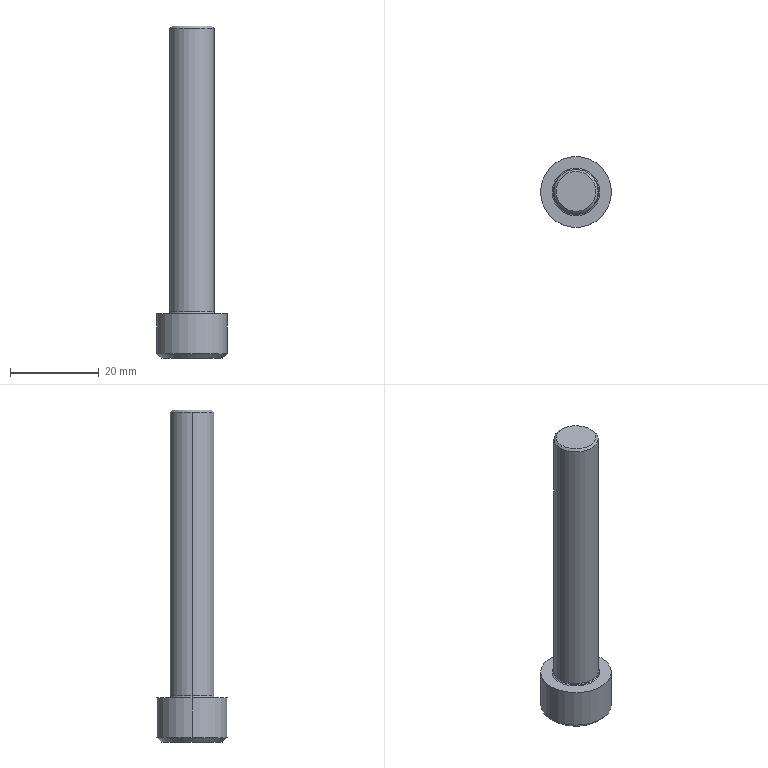Part | Creo | 1 solid | 23 faces | box 16 x 16 x 75 mm | volume 6754 mm3 | plane 9 | cone 6 | cylinder 4 | torus 4 | commonest cylinder face diameters 10 x2 16 x2
STEP:
#1=CARTESIAN_POINT('',(232.817,-87.997,-4.));
#2=VERTEX_POINT('',#1);
#3=CARTESIAN_POINT('',(235.126,-83.997,-4.));
#4=VERTEX_POINT('',#3);
#5=CARTESIAN_POINT('',(232.817,-87.997,-4.));
#6=CARTESIAN_POINT('',(232.943,-87.779,-3.928));
#7=CARTESIAN_POINT('',(233.195,-87.342,-3.799));
#8=CARTESIAN_POINT('',(233.581,-86.674,-3.673));
#9=CARTESIAN_POINT('',(233.971,-85.999,-3.628));
#10=CARTESIAN_POINT('',(234.362,-85.321,-3.672));
#11=CARTESIAN_POINT('',(234.747,-84.654,-3.799));
#12=CARTESIAN_POINT('',(235.,-84.215,-3.927));
#13=CARTESIAN_POINT('',(235.126,-83.997,-4.));
#14=B_SPLINE_CURVE_WITH_KNOTS('',3,(#5,#6,#7,#8,#9,#10,#11,#12,#13),.UNSPECIFIED.,.F.,.F.,(4,1,1,1,1,1,4),(0.,0.1667,0.3333,0.5,0.6667,0.8333,1.),.UNSPECIFIED.);
#15=EDGE_CURVE('',#2,#4,#14,.T.);
#16=ORIENTED_EDGE('',*,*,#15,.F.);
#17=CARTESIAN_POINT('',(237.436,-87.997,-1.333));
#18=VERTEX_POINT('',#17);
#19=CARTESIAN_POINT('',(237.436,-87.997,-1.333));
#20=DIRECTION('',(-0.866,0.,-0.5));
#21=VECTOR('',#20,5.333);
#22=LINE('',#19,#21);
#23=EDGE_CURVE('',#18,#2,#22,.T.);
#24=ORIENTED_EDGE('',*,*,#23,.F.);
#25=CARTESIAN_POINT('',(242.055,-87.997,-4.));
#26=VERTEX_POINT('',#25);
#27=CARTESIAN_POINT('',(237.436,-87.997,-1.333));
#28=DIRECTION('',(0.866,0.,-0.5));
#29=VECTOR('',#28,5.333);
#30=LINE('',#27,#29);
#31=EDGE_CURVE('',#18,#26,#30,.T.);
#32=ORIENTED_EDGE('',*,*,#31,.T.);
#33=CARTESIAN_POINT('',(239.745,-83.997,-4.));
#34=VERTEX_POINT('',#33);
#35=CARTESIAN_POINT('',(239.745,-83.997,-4.));
#36=CARTESIAN_POINT('',(239.871,-84.214,-3.928));
#37=CARTESIAN_POINT('',(240.123,-84.651,-3.799));
#38=CARTESIAN_POINT('',(240.509,-85.32,-3.673));
#39=CARTESIAN_POINT('',(240.899,-85.995,-3.628));
#40=CARTESIAN_POINT('',(241.29,-86.673,-3.672));
#41=CARTESIAN_POINT('',(241.675,-87.34,-3.799));
#42=CARTESIAN_POINT('',(241.929,-87.778,-3.927));
#43=CARTESIAN_POINT('',(242.055,-87.997,-4.));
#44=B_SPLINE_CURVE_WITH_KNOTS('',3,(#35,#36,#37,#38,#39,#40,#41,#42,#43),.UNSPECIFIED.,.F.,.F.,(4,1,1,1,1,1,4),(0.,0.1667,0.3333,0.5,0.6667,0.8333,1.),.UNSPECIFIED.);
#45=EDGE_CURVE('',#34,#26,#44,.T.);
#46=ORIENTED_EDGE('',*,*,#45,.F.);
#47=CARTESIAN_POINT('',(235.126,-83.997,-4.));
#48=CARTESIAN_POINT('',(235.376,-83.997,-3.928));
#49=CARTESIAN_POINT('',(235.88,-83.997,-3.8));
#50=CARTESIAN_POINT('',(236.654,-83.997,-3.673));
#51=CARTESIAN_POINT('',(237.435,-83.997,-3.628));
#52=CARTESIAN_POINT('',(238.215,-83.997,-3.672));
#53=CARTESIAN_POINT('',(238.988,-83.997,-3.799));
#54=CARTESIAN_POINT('',(239.494,-83.997,-3.927));
#55=CARTESIAN_POINT('',(239.745,-83.997,-4.));
#56=B_SPLINE_CURVE_WITH_KNOTS('',3,(#47,#48,#49,#50,#51,#52,#53,#54,#55),.UNSPECIFIED.,.F.,.F.,(4,1,1,1,1,1,4),(0.,0.1667,0.3333,0.5,0.6667,0.8333,1.),.UNSPECIFIED.);
#57=EDGE_CURVE('',#4,#34,#56,.T.);
#58=ORIENTED_EDGE('',*,*,#57,.F.);
#59=EDGE_LOOP('',(#16,#24,#32,#46,#58));
#60=FACE_OUTER_BOUND('',#59,.F.);
#61=CARTESIAN_POINT('',(237.436,-87.997,-2.693));
#62=DIRECTION('',(0.,0.,-1.));
#63=DIRECTION('',(-1.,0.,0.));
#64=AXIS2_PLACEMENT_3D('',#61,#62,#63);
#65=CONICAL_SURFACE('',#64,2.356,60.);
#66=ADVANCED_FACE('',(#60),#65,.F.);
#67=CARTESIAN_POINT('',(235.126,-83.997,-9.));
#68=VERTEX_POINT('',#67);
#69=CARTESIAN_POINT('',(232.817,-87.997,-9.));
#70=VERTEX_POINT('',#69);
#71=CARTESIAN_POINT('',(235.126,-83.997,-9.));
#72=DIRECTION('',(-0.5,-0.866,0.));
#73=VECTOR('',#72,4.619);
#74=LINE('',#71,#73);
#75=EDGE_CURVE('',#68,#70,#74,.T.);
#76=ORIENTED_EDGE('',*,*,#75,.T.);
#77=CARTESIAN_POINT('',(232.817,-87.997,-9.));
#78=DIRECTION('',(0.,0.,1.));
#79=VECTOR('',#78,5.);
#80=LINE('',#77,#79);
#81=EDGE_CURVE('',#70,#2,#80,.T.);
#82=ORIENTED_EDGE('',*,*,#81,.T.);
#83=ORIENTED_EDGE('',*,*,#15,.T.);
#84=CARTESIAN_POINT('',(235.126,-83.997,-9.));
#85=DIRECTION('',(0.,0.,1.));
#86=VECTOR('',#85,5.);
#87=LINE('',#84,#86);
#88=EDGE_CURVE('',#68,#4,#87,.T.);
#89=ORIENTED_EDGE('',*,*,#88,.F.);
#90=EDGE_LOOP('',(#76,#82,#83,#89));
#91=FACE_OUTER_BOUND('',#90,.F.);
#92=CARTESIAN_POINT('',(235.126,-83.997,-4.));
#93=DIRECTION('',(0.866,-0.5,0.));
#94=DIRECTION('',(-0.5,-0.866,0.));
#95=AXIS2_PLACEMENT_3D('',#92,#93,#94);
#96=PLANE('',#95);
#97=ADVANCED_FACE('',(#91),#96,.T.);
#98=CARTESIAN_POINT('',(230.436,-87.997,-9.));
#99=VERTEX_POINT('',#98);
#100=CARTESIAN_POINT('',(244.436,-87.997,-9.));
#101=VERTEX_POINT('',#100);
#102=CARTESIAN_POINT('',(237.436,-87.997,-9.));
#103=DIRECTION('',(0.,0.,-1.));
#104=DIRECTION('',(-1.,0.,0.));
#105=AXIS2_PLACEMENT_3D('',#102,#103,#104);
#106=CIRCLE('',#105,7.);
#107=EDGE_CURVE('',#99,#101,#106,.T.);
#108=ORIENTED_EDGE('',*,*,#107,.F.);
#109=CARTESIAN_POINT('',(237.436,-87.997,-9.));
#110=DIRECTION('',(0.,0.,-1.));
#111=DIRECTION('',(1.,0.,0.));
#112=AXIS2_PLACEMENT_3D('',#109,#110,#111);
#113=CIRCLE('',#112,7.);
#114=EDGE_CURVE('',#101,#99,#113,.T.);
#115=ORIENTED_EDGE('',*,*,#114,.F.);
#116=EDGE_LOOP('',(#108,#115));
#117=FACE_OUTER_BOUND('',#116,.F.);
#118=CARTESIAN_POINT('',(235.126,-91.997,-9.));
#119=VERTEX_POINT('',#118);
#120=CARTESIAN_POINT('',(232.817,-87.997,-9.));
#121=DIRECTION('',(0.5,-0.866,0.));
#122=VECTOR('',#121,4.619);
#123=LINE('',#120,#122);
#124=EDGE_CURVE('',#70,#119,#123,.T.);
#125=ORIENTED_EDGE('',*,*,#124,.F.);
#126=ORIENTED_EDGE('',*,*,#75,.F.);
#127=CARTESIAN_POINT('',(239.745,-83.997,-9.));
#128=VERTEX_POINT('',#127);
#129=CARTESIAN_POINT('',(235.126,-83.997,-9.));
#130=DIRECTION('',(1.,0.,0.));
#131=VECTOR('',#130,4.619);
#132=LINE('',#129,#131);
#133=EDGE_CURVE('',#68,#128,#132,.T.);
#134=ORIENTED_EDGE('',*,*,#133,.T.);
#135=CARTESIAN_POINT('',(242.055,-87.997,-9.));
#136=VERTEX_POINT('',#135);
#137=CARTESIAN_POINT('',(242.055,-87.997,-9.));
#138=DIRECTION('',(-0.5,0.866,0.));
#139=VECTOR('',#138,4.619);
#140=LINE('',#137,#139);
#141=EDGE_CURVE('',#136,#128,#140,.T.);
#142=ORIENTED_EDGE('',*,*,#141,.F.);
#143=CARTESIAN_POINT('',(239.745,-91.997,-9.));
#144=VERTEX_POINT('',#143);
#145=CARTESIAN_POINT('',(239.745,-91.997,-9.));
#146=DIRECTION('',(0.5,0.866,0.));
#147=VECTOR('',#146,4.619);
#148=LINE('',#145,#147);
#149=EDGE_CURVE('',#144,#136,#148,.T.);
#150=ORIENTED_EDGE('',*,*,#149,.F.);
#151=CARTESIAN_POINT('',(239.745,-91.997,-9.));
#152=DIRECTION('',(-1.,0.,0.));
#153=VECTOR('',#152,4.619);
#154=LINE('',#151,#153);
#155=EDGE_CURVE('',#144,#119,#154,.T.);
#156=ORIENTED_EDGE('',*,*,#155,.T.);
#157=EDGE_LOOP('',(#125,#126,#134,#142,#150,#156));
#158=FACE_BOUND('',#157,.F.);
#159=CARTESIAN_POINT('',(237.436,-87.997,-9.));
#160=DIRECTION('',(0.,0.,-1.));
#161=DIRECTION('',(-1.,0.,0.));
#162=AXIS2_PLACEMENT_3D('',#159,#160,#161);
#163=PLANE('',#162);
#164=ADVANCED_FACE('',(#117,#158),#163,.T.);
#165=CARTESIAN_POINT('',(229.436,-87.997,-8.));
#166=VERTEX_POINT('',#165);
#167=CARTESIAN_POINT('',(245.436,-87.997,-8.));
#168=VERTEX_POINT('',#167);
#169=CARTESIAN_POINT('',(237.436,-87.997,-8.));
#170=DIRECTION('',(0.,0.,-1.));
#171=DIRECTION('',(-1.,0.,0.));
#172=AXIS2_PLACEMENT_3D('',#169,#170,#171);
#173=CIRCLE('',#172,8.);
#174=EDGE_CURVE('',#166,#168,#173,.T.);
#175=ORIENTED_EDGE('',*,*,#174,.F.);
#176=CARTESIAN_POINT('',(230.436,-87.997,-9.));
#177=DIRECTION('',(-0.7071,0.,0.7071));
#178=VECTOR('',#177,1.414);
#179=LINE('',#176,#178);
#180=EDGE_CURVE('',#99,#166,#179,.T.);
#181=ORIENTED_EDGE('',*,*,#180,.F.);
#182=ORIENTED_EDGE('',*,*,#107,.T.);
#183=CARTESIAN_POINT('',(244.436,-87.997,-9.));
#184=DIRECTION('',(0.7071,0.,0.7071));
#185=VECTOR('',#184,1.414);
#186=LINE('',#183,#185);
#187=EDGE_CURVE('',#101,#168,#186,.T.);
#188=ORIENTED_EDGE('',*,*,#187,.T.);
#189=EDGE_LOOP('',(#175,#181,#182,#188));
#190=FACE_OUTER_BOUND('',#189,.F.);
#191=CARTESIAN_POINT('',(237.436,-87.997,-8.5));
#192=DIRECTION('',(0.,0.,1.));
#193=DIRECTION('',(1.,0.,0.));
#194=AXIS2_PLACEMENT_3D('',#191,#192,#193);
#195=CONICAL_SURFACE('',#194,7.5,45.);
#196=ADVANCED_FACE('',(#190),#195,.T.);
#197=ORIENTED_EDGE('',*,*,#174,.T.);
#198=CARTESIAN_POINT('',(245.436,-87.997,0.9999));
#199=VERTEX_POINT('',#198);
#200=CARTESIAN_POINT('',(245.436,-87.997,0.9999));
#201=DIRECTION('',(0.,0.,-1.));
#202=VECTOR('',#201,9.);
#203=LINE('',#200,#202);
#204=EDGE_CURVE('',#199,#168,#203,.T.);
#205=ORIENTED_EDGE('',*,*,#204,.F.);
#206=CARTESIAN_POINT('',(229.436,-87.997,0.9999));
#207=VERTEX_POINT('',#206);
#208=CARTESIAN_POINT('',(237.436,-87.997,0.9999));
#209=DIRECTION('',(0.,0.,1.));
#210=DIRECTION('',(1.,0.,0.));
#211=AXIS2_PLACEMENT_3D('',#208,#209,#210);
#212=CIRCLE('',#211,8.);
#213=EDGE_CURVE('',#199,#207,#212,.T.);
#214=ORIENTED_EDGE('',*,*,#213,.T.);
#215=CARTESIAN_POINT('',(229.436,-87.997,0.9999));
#216=DIRECTION('',(0.,0.,-1.));
#217=VECTOR('',#216,9.);
#218=LINE('',#215,#217);
#219=EDGE_CURVE('',#207,#166,#218,.T.);
#220=ORIENTED_EDGE('',*,*,#219,.T.);
#221=EDGE_LOOP('',(#197,#205,#214,#220));
#222=FACE_OUTER_BOUND('',#221,.F.);
#223=CARTESIAN_POINT('',(237.436,-87.997,0.9999));
#224=DIRECTION('',(0.,0.,-1.));
#225=DIRECTION('',(-1.,0.,0.));
#226=AXIS2_PLACEMENT_3D('',#223,#224,#225);
#227=CYLINDRICAL_SURFACE('',#226,8.);
#228=ADVANCED_FACE('',(#222),#227,.T.);
#229=CARTESIAN_POINT('',(237.436,-87.997,-8.));
#230=DIRECTION('',(0.,0.,-1.));
#231=DIRECTION('',(1.,0.,0.));
#232=AXIS2_PLACEMENT_3D('',#229,#230,#231);
#233=CIRCLE('',#232,8.);
#234=EDGE_CURVE('',#168,#166,#233,.T.);
#235=ORIENTED_EDGE('',*,*,#234,.T.);
#236=ORIENTED_EDGE('',*,*,#219,.F.);
#237=CARTESIAN_POINT('',(237.436,-87.997,0.9999));
#238=DIRECTION('',(0.,0.,1.));
#239=DIRECTION('',(-1.,0.,0.));
#240=AXIS2_PLACEMENT_3D('',#237,#238,#239);
#241=CIRCLE('',#240,8.);
#242=EDGE_CURVE('',#207,#199,#241,.T.);
#243=ORIENTED_EDGE('',*,*,#242,.T.);
#244=ORIENTED_EDGE('',*,*,#204,.T.);
#245=EDGE_LOOP('',(#235,#236,#243,#244));
#246=FACE_OUTER_BOUND('',#245,.F.);
#247=CARTESIAN_POINT('',(237.436,-87.997,0.9999));
#248=DIRECTION('',(0.,0.,-1.));
#249=DIRECTION('',(-1.,0.,0.));
#250=AXIS2_PLACEMENT_3D('',#247,#248,#249);
#251=CYLINDRICAL_SURFACE('',#250,8.);
#252=ADVANCED_FACE('',(#246),#251,.T.);
#253=ORIENTED_EDGE('',*,*,#234,.F.);
#254=ORIENTED_EDGE('',*,*,#187,.F.);
#255=ORIENTED_EDGE('',*,*,#114,.T.);
#256=ORIENTED_EDGE('',*,*,#180,.T.);
#257=EDGE_LOOP('',(#253,#254,#255,#256));
#258=FACE_OUTER_BOUND('',#257,.F.);
#259=CARTESIAN_POINT('',(237.436,-87.997,-8.5));
#260=DIRECTION('',(0.,0.,1.));
#261=DIRECTION('',(1.,0.,0.));
#262=AXIS2_PLACEMENT_3D('',#259,#260,#261);
#263=CONICAL_SURFACE('',#262,7.5,45.);
#264=ADVANCED_FACE('',(#258),#263,.T.);
#265=ORIENTED_EDGE('',*,*,#242,.F.);
#266=ORIENTED_EDGE('',*,*,#213,.F.);
#267=EDGE_LOOP('',(#265,#266));
#268=FACE_OUTER_BOUND('',#267,.F.);
#269=CARTESIAN_POINT('',(232.036,-87.997,0.9999));
#270=VERTEX_POINT('',#269);
#271=CARTESIAN_POINT('',(242.836,-87.997,0.9999));
#272=VERTEX_POINT('',#271);
#273=CARTESIAN_POINT('',(237.436,-87.997,0.9999));
#274=DIRECTION('',(0.,0.,-1.));
#275=DIRECTION('',(-1.,0.,0.));
#276=AXIS2_PLACEMENT_3D('',#273,#274,#275);
#277=CIRCLE('',#276,5.4);
#278=EDGE_CURVE('',#270,#272,#277,.T.);
#279=ORIENTED_EDGE('',*,*,#278,.F.);
#280=CARTESIAN_POINT('',(237.436,-87.997,0.9999));
#281=DIRECTION('',(0.,0.,-1.));
#282=DIRECTION('',(1.,0.,0.));
#283=AXIS2_PLACEMENT_3D('',#280,#281,#282);
#284=CIRCLE('',#283,5.4);
#285=EDGE_CURVE('',#272,#270,#284,.T.);
#286=ORIENTED_EDGE('',*,*,#285,.F.);
#287=EDGE_LOOP('',(#279,#286));
#288=FACE_BOUND('',#287,.F.);
#289=CARTESIAN_POINT('',(237.436,-87.997,0.9999));
#290=DIRECTION('',(0.,0.,-1.));
#291=DIRECTION('',(-1.,0.,0.));
#292=AXIS2_PLACEMENT_3D('',#289,#290,#291);
#293=PLANE('',#292);
#294=ADVANCED_FACE('',(#268,#288),#293,.F.);
#295=ORIENTED_EDGE('',*,*,#278,.T.);
#296=CARTESIAN_POINT('',(242.553,-87.997,1.117));
#297=VERTEX_POINT('',#296);
#298=CARTESIAN_POINT('',(242.836,-87.997,1.4));
#299=DIRECTION('',(0.,1.,0.));
#300=DIRECTION('',(0.,0.,-1.));
#301=AXIS2_PLACEMENT_3D('',#298,#299,#300);
#302=CIRCLE('',#301,0.4);
#303=EDGE_CURVE('',#272,#297,#302,.T.);
#304=ORIENTED_EDGE('',*,*,#303,.T.);
#305=CARTESIAN_POINT('',(232.319,-87.997,1.117));
#306=VERTEX_POINT('',#305);
#307=CARTESIAN_POINT('',(237.436,-87.997,1.117));
#308=DIRECTION('',(0.,0.,-1.));
#309=DIRECTION('',(-1.,0.,0.));
#310=AXIS2_PLACEMENT_3D('',#307,#308,#309);
#311=CIRCLE('',#310,5.117);
#312=EDGE_CURVE('',#306,#297,#311,.T.);
#313=ORIENTED_EDGE('',*,*,#312,.F.);
#314=CARTESIAN_POINT('',(232.036,-87.997,1.4));
#315=DIRECTION('',(0.,-1.,0.));
#316=DIRECTION('',(0.,0.,-1.));
#317=AXIS2_PLACEMENT_3D('',#314,#315,#316);
#318=CIRCLE('',#317,0.4);
#319=EDGE_CURVE('',#270,#306,#318,.T.);
#320=ORIENTED_EDGE('',*,*,#319,.F.);
#321=EDGE_LOOP('',(#295,#304,#313,#320));
#322=FACE_OUTER_BOUND('',#321,.F.);
#323=CARTESIAN_POINT('',(237.436,-87.997,1.4));
#324=DIRECTION('',(0.,0.,-1.));
#325=DIRECTION('',(-1.,0.,0.));
#326=AXIS2_PLACEMENT_3D('',#323,#324,#325);
#327=TOROIDAL_SURFACE('',#326,5.4,0.4);
#328=ADVANCED_FACE('',(#322),#327,.F.);
#329=ORIENTED_EDGE('',*,*,#285,.T.);
#330=ORIENTED_EDGE('',*,*,#319,.T.);
#331=CARTESIAN_POINT('',(237.436,-87.997,1.117));
#332=DIRECTION('',(0.,0.,-1.));
#333=DIRECTION('',(1.,0.,0.));
#334=AXIS2_PLACEMENT_3D('',#331,#332,#333);
#335=CIRCLE('',#334,5.117);
#336=EDGE_CURVE('',#297,#306,#335,.T.);
#337=ORIENTED_EDGE('',*,*,#336,.F.);
#338=ORIENTED_EDGE('',*,*,#303,.F.);
#339=EDGE_LOOP('',(#329,#330,#337,#338));
#340=FACE_OUTER_BOUND('',#339,.F.);
#341=CARTESIAN_POINT('',(237.436,-87.997,1.4));
#342=DIRECTION('',(0.,0.,-1.));
#343=DIRECTION('',(-1.,0.,0.));
#344=AXIS2_PLACEMENT_3D('',#341,#342,#343);
#345=TOROIDAL_SURFACE('',#344,5.4,0.4);
#346=ADVANCED_FACE('',(#340),#345,.F.);
#347=CARTESIAN_POINT('',(242.436,-87.997,1.4));
#348=VERTEX_POINT('',#347);
#349=CARTESIAN_POINT('',(232.436,-87.997,1.4));
#350=VERTEX_POINT('',#349);
#351=CARTESIAN_POINT('',(237.436,-87.997,1.4));
#352=DIRECTION('',(0.,0.,-1.));
#353=DIRECTION('',(1.,0.,0.));
#354=AXIS2_PLACEMENT_3D('',#351,#352,#353);
#355=CIRCLE('',#354,5.);
#356=EDGE_CURVE('',#348,#350,#355,.T.);
#357=ORIENTED_EDGE('',*,*,#356,.F.);
#358=CARTESIAN_POINT('',(242.836,-87.997,1.4));
#359=DIRECTION('',(0.,1.,0.));
#360=DIRECTION('',(-0.7071,0.,-0.7071));
#361=AXIS2_PLACEMENT_3D('',#358,#359,#360);
#362=CIRCLE('',#361,0.4);
#363=EDGE_CURVE('',#297,#348,#362,.T.);
#364=ORIENTED_EDGE('',*,*,#363,.F.);
#365=ORIENTED_EDGE('',*,*,#336,.T.);
#366=CARTESIAN_POINT('',(232.036,-87.997,1.4));
#367=DIRECTION('',(0.,-1.,0.));
#368=DIRECTION('',(0.7071,0.,-0.7071));
#369=AXIS2_PLACEMENT_3D('',#366,#367,#368);
#370=CIRCLE('',#369,0.4);
#371=EDGE_CURVE('',#306,#350,#370,.T.);
#372=ORIENTED_EDGE('',*,*,#371,.T.);
#373=EDGE_LOOP('',(#357,#364,#365,#372));
#374=FACE_OUTER_BOUND('',#373,.F.);
#375=CARTESIAN_POINT('',(237.436,-87.997,1.4));
#376=DIRECTION('',(0.,0.,-1.));
#377=DIRECTION('',(-1.,0.,0.));
#378=AXIS2_PLACEMENT_3D('',#375,#376,#377);
#379=TOROIDAL_SURFACE('',#378,5.4,0.4);
#380=ADVANCED_FACE('',(#374),#379,.F.);
#381=CARTESIAN_POINT('',(232.436,-87.997,65.5));
#382=VERTEX_POINT('',#381);
#383=CARTESIAN_POINT('',(242.436,-87.997,65.5));
#384=VERTEX_POINT('',#383);
#385=CARTESIAN_POINT('',(237.436,-87.997,65.5));
#386=DIRECTION('',(0.,0.,1.));
#387=DIRECTION('',(-1.,0.,0.));
#388=AXIS2_PLACEMENT_3D('',#385,#386,#387);
#389=CIRCLE('',#388,5.);
#390=EDGE_CURVE('',#382,#384,#389,.T.);
#391=ORIENTED_EDGE('',*,*,#390,.T.);
#392=CARTESIAN_POINT('',(242.436,-87.997,65.5));
#393=DIRECTION('',(0.,0.,-1.));
#394=VECTOR('',#393,64.1);
#395=LINE('',#392,#394);
#396=EDGE_CURVE('',#384,#348,#395,.T.);
#397=ORIENTED_EDGE('',*,*,#396,.T.);
#398=ORIENTED_EDGE('',*,*,#356,.T.);
#399=CARTESIAN_POINT('',(232.436,-87.997,65.5));
#400=DIRECTION('',(0.,0.,-1.));
#401=VECTOR('',#400,64.1);
#402=LINE('',#399,#401);
#403=EDGE_CURVE('',#382,#350,#402,.T.);
#404=ORIENTED_EDGE('',*,*,#403,.F.);
#405=EDGE_LOOP('',(#391,#397,#398,#404));
#406=FACE_OUTER_BOUND('',#405,.F.);
#407=CARTESIAN_POINT('',(237.436,-87.997,66.));
#408=DIRECTION('',(0.,0.,-1.));
#409=DIRECTION('',(-1.,0.,0.));
#410=AXIS2_PLACEMENT_3D('',#407,#408,#409);
#411=CYLINDRICAL_SURFACE('',#410,5.);
#412=ADVANCED_FACE('',(#406),#411,.T.);
#413=CARTESIAN_POINT('',(232.936,-87.997,66.));
#414=VERTEX_POINT('',#413);
#415=CARTESIAN_POINT('',(241.936,-87.997,66.));
#416=VERTEX_POINT('',#415);
#417=CARTESIAN_POINT('',(237.436,-87.997,66.));
#418=DIRECTION('',(0.,0.,1.));
#419=DIRECTION('',(-1.,0.,0.));
#420=AXIS2_PLACEMENT_3D('',#417,#418,#419);
#421=CIRCLE('',#420,4.5);
#422=EDGE_CURVE('',#414,#416,#421,.T.);
#423=ORIENTED_EDGE('',*,*,#422,.T.);
#424=CARTESIAN_POINT('',(241.936,-87.997,66.));
#425=DIRECTION('',(0.7071,0.,-0.7071));
#426=VECTOR('',#425,0.7071);
#427=LINE('',#424,#426);
#428=EDGE_CURVE('',#416,#384,#427,.T.);
#429=ORIENTED_EDGE('',*,*,#428,.T.);
#430=ORIENTED_EDGE('',*,*,#390,.F.);
#431=CARTESIAN_POINT('',(232.936,-87.997,66.));
#432=DIRECTION('',(-0.7071,0.,-0.7071));
#433=VECTOR('',#432,0.7071);
#434=LINE('',#431,#433);
#435=EDGE_CURVE('',#414,#382,#434,.T.);
#436=ORIENTED_EDGE('',*,*,#435,.F.);
#437=EDGE_LOOP('',(#423,#429,#430,#436));
#438=FACE_OUTER_BOUND('',#437,.F.);
#439=CARTESIAN_POINT('',(237.436,-87.997,65.75));
#440=DIRECTION('',(0.,0.,-1.));
#441=DIRECTION('',(-1.,0.,0.));
#442=AXIS2_PLACEMENT_3D('',#439,#440,#441);
#443=CONICAL_SURFACE('',#442,4.75,45.);
#444=ADVANCED_FACE('',(#438),#443,.T.);
#445=ORIENTED_EDGE('',*,*,#422,.F.);
#446=CARTESIAN_POINT('',(237.436,-87.997,66.));
#447=DIRECTION('',(0.,0.,1.));
#448=DIRECTION('',(1.,0.,0.));
#449=AXIS2_PLACEMENT_3D('',#446,#447,#448);
#450=CIRCLE('',#449,4.5);
#451=EDGE_CURVE('',#416,#414,#450,.T.);
#452=ORIENTED_EDGE('',*,*,#451,.F.);
#453=EDGE_LOOP('',(#445,#452));
#454=FACE_OUTER_BOUND('',#453,.F.);
#455=CARTESIAN_POINT('',(237.436,-87.997,66.));
#456=DIRECTION('',(0.,0.,-1.));
#457=DIRECTION('',(-1.,0.,0.));
#458=AXIS2_PLACEMENT_3D('',#455,#456,#457);
#459=PLANE('',#458);
#460=ADVANCED_FACE('',(#454),#459,.F.);
#461=ORIENTED_EDGE('',*,*,#451,.T.);
#462=ORIENTED_EDGE('',*,*,#435,.T.);
#463=CARTESIAN_POINT('',(237.436,-87.997,65.5));
#464=DIRECTION('',(0.,0.,1.));
#465=DIRECTION('',(1.,0.,0.));
#466=AXIS2_PLACEMENT_3D('',#463,#464,#465);
#467=CIRCLE('',#466,5.);
#468=EDGE_CURVE('',#384,#382,#467,.T.);
#469=ORIENTED_EDGE('',*,*,#468,.F.);
#470=ORIENTED_EDGE('',*,*,#428,.F.);
#471=EDGE_LOOP('',(#461,#462,#469,#470));
#472=FACE_OUTER_BOUND('',#471,.F.);
#473=CARTESIAN_POINT('',(237.436,-87.997,65.75));
#474=DIRECTION('',(0.,0.,-1.));
#475=DIRECTION('',(-1.,0.,0.));
#476=AXIS2_PLACEMENT_3D('',#473,#474,#475);
#477=CONICAL_SURFACE('',#476,4.75,45.);
#478=ADVANCED_FACE('',(#472),#477,.T.);
#479=ORIENTED_EDGE('',*,*,#468,.T.);
#480=ORIENTED_EDGE('',*,*,#403,.T.);
#481=CARTESIAN_POINT('',(237.436,-87.997,1.4));
#482=DIRECTION('',(0.,0.,-1.));
#483=DIRECTION('',(-1.,0.,0.));
#484=AXIS2_PLACEMENT_3D('',#481,#482,#483);
#485=CIRCLE('',#484,5.);
#486=EDGE_CURVE('',#350,#348,#485,.T.);
#487=ORIENTED_EDGE('',*,*,#486,.T.);
#488=ORIENTED_EDGE('',*,*,#396,.F.);
#489=EDGE_LOOP('',(#479,#480,#487,#488));
#490=FACE_OUTER_BOUND('',#489,.F.);
#491=CARTESIAN_POINT('',(237.436,-87.997,66.));
#492=DIRECTION('',(0.,0.,-1.));
#493=DIRECTION('',(-1.,0.,0.));
#494=AXIS2_PLACEMENT_3D('',#491,#492,#493);
#495=CYLINDRICAL_SURFACE('',#494,5.);
#496=ADVANCED_FACE('',(#490),#495,.T.);
#497=ORIENTED_EDGE('',*,*,#486,.F.);
#498=ORIENTED_EDGE('',*,*,#371,.F.);
#499=ORIENTED_EDGE('',*,*,#312,.T.);
#500=ORIENTED_EDGE('',*,*,#363,.T.);
#501=EDGE_LOOP('',(#497,#498,#499,#500));
#502=FACE_OUTER_BOUND('',#501,.F.);
#503=CARTESIAN_POINT('',(237.436,-87.997,1.4));
#504=DIRECTION('',(0.,0.,-1.));
#505=DIRECTION('',(-1.,0.,0.));
#506=AXIS2_PLACEMENT_3D('',#503,#504,#505);
#507=TOROIDAL_SURFACE('',#506,5.4,0.4);
#508=ADVANCED_FACE('',(#502),#507,.F.);
#509=ORIENTED_EDGE('',*,*,#124,.T.);
#510=CARTESIAN_POINT('',(235.126,-91.997,-4.));
#511=VERTEX_POINT('',#510);
#512=CARTESIAN_POINT('',(235.126,-91.997,-9.));
#513=DIRECTION('',(0.,0.,1.));
#514=VECTOR('',#513,5.);
#515=LINE('',#512,#514);
#516=EDGE_CURVE('',#119,#511,#515,.T.);
#517=ORIENTED_EDGE('',*,*,#516,.T.);
#518=CARTESIAN_POINT('',(235.126,-91.997,-4.));
#519=CARTESIAN_POINT('',(235.001,-91.779,-3.928));
#520=CARTESIAN_POINT('',(234.749,-91.342,-3.799));
#521=CARTESIAN_POINT('',(234.363,-90.674,-3.673));
#522=CARTESIAN_POINT('',(233.973,-89.999,-3.628));
#523=CARTESIAN_POINT('',(233.582,-89.321,-3.672));
#524=CARTESIAN_POINT('',(233.196,-88.654,-3.799));
#525=CARTESIAN_POINT('',(232.943,-88.215,-3.927));
#526=CARTESIAN_POINT('',(232.817,-87.997,-4.));
#527=B_SPLINE_CURVE_WITH_KNOTS('',3,(#518,#519,#520,#521,#522,#523,#524,#525,#526),.UNSPECIFIED.,.F.,.F.,(4,1,1,1,1,1,4),(0.,0.1667,0.3333,0.5,0.6667,0.8333,1.),.UNSPECIFIED.);
#528=EDGE_CURVE('',#511,#2,#527,.T.);
#529=ORIENTED_EDGE('',*,*,#528,.T.);
#530=ORIENTED_EDGE('',*,*,#81,.F.);
#531=EDGE_LOOP('',(#509,#517,#529,#530));
#532=FACE_OUTER_BOUND('',#531,.F.);
#533=CARTESIAN_POINT('',(232.817,-87.997,-4.));
#534=DIRECTION('',(0.866,0.5,0.));
#535=DIRECTION('',(0.5,-0.866,0.));
#536=AXIS2_PLACEMENT_3D('',#533,#534,#535);
#537=PLANE('',#536);
#538=ADVANCED_FACE('',(#532),#537,.T.);
#539=ORIENTED_EDGE('',*,*,#155,.F.);
#540=CARTESIAN_POINT('',(239.745,-91.997,-4.));
#541=VERTEX_POINT('',#540);
#542=CARTESIAN_POINT('',(239.745,-91.997,-9.));
#543=DIRECTION('',(0.,0.,1.));
#544=VECTOR('',#543,5.);
#545=LINE('',#542,#544);
#546=EDGE_CURVE('',#144,#541,#545,.T.);
#547=ORIENTED_EDGE('',*,*,#546,.T.);
#548=CARTESIAN_POINT('',(239.745,-91.997,-4.));
#549=CARTESIAN_POINT('',(239.494,-91.997,-3.927));
#550=CARTESIAN_POINT('',(238.988,-91.997,-3.799));
#551=CARTESIAN_POINT('',(238.215,-91.997,-3.672));
#552=CARTESIAN_POINT('',(237.435,-91.997,-3.628));
#553=CARTESIAN_POINT('',(236.654,-91.997,-3.673));
#554=CARTESIAN_POINT('',(235.88,-91.997,-3.8));
#555=CARTESIAN_POINT('',(235.376,-91.997,-3.928));
#556=CARTESIAN_POINT('',(235.126,-91.997,-4.));
#557=B_SPLINE_CURVE_WITH_KNOTS('',3,(#548,#549,#550,#551,#552,#553,#554,#555,#556),.UNSPECIFIED.,.F.,.F.,(4,1,1,1,1,1,4),(0.,0.1667,0.3333,0.5,0.6667,0.8333,1.),.UNSPECIFIED.);
#558=EDGE_CURVE('',#541,#511,#557,.T.);
#559=ORIENTED_EDGE('',*,*,#558,.T.);
#560=ORIENTED_EDGE('',*,*,#516,.F.);
#561=EDGE_LOOP('',(#539,#547,#559,#560));
#562=FACE_OUTER_BOUND('',#561,.F.);
#563=CARTESIAN_POINT('',(235.126,-91.997,-4.));
#564=DIRECTION('',(0.,1.,0.));
#565=DIRECTION('',(0.,0.,-1.));
#566=AXIS2_PLACEMENT_3D('',#563,#564,#565);
#567=PLANE('',#566);
#568=ADVANCED_FACE('',(#562),#567,.T.);
#569=ORIENTED_EDGE('',*,*,#149,.T.);
#570=CARTESIAN_POINT('',(242.055,-87.997,-9.));
#571=DIRECTION('',(0.,0.,1.));
#572=VECTOR('',#571,5.);
#573=LINE('',#570,#572);
#574=EDGE_CURVE('',#136,#26,#573,.T.);
#575=ORIENTED_EDGE('',*,*,#574,.T.);
#576=CARTESIAN_POINT('',(242.055,-87.997,-4.));
#577=CARTESIAN_POINT('',(241.929,-88.215,-3.927));
#578=CARTESIAN_POINT('',(241.675,-88.654,-3.799));
#579=CARTESIAN_POINT('',(241.29,-89.321,-3.672));
#580=CARTESIAN_POINT('',(240.899,-89.999,-3.628));
#581=CARTESIAN_POINT('',(240.509,-90.674,-3.673));
#582=CARTESIAN_POINT('',(240.123,-91.342,-3.799));
#583=CARTESIAN_POINT('',(239.871,-91.779,-3.928));
#584=CARTESIAN_POINT('',(239.745,-91.997,-4.));
#585=B_SPLINE_CURVE_WITH_KNOTS('',3,(#576,#577,#578,#579,#580,#581,#582,#583,#584),.UNSPECIFIED.,.F.,.F.,(4,1,1,1,1,1,4),(0.,0.1667,0.3333,0.5,0.6667,0.8333,1.),.UNSPECIFIED.);
#586=EDGE_CURVE('',#26,#541,#585,.T.);
#587=ORIENTED_EDGE('',*,*,#586,.T.);
#588=ORIENTED_EDGE('',*,*,#546,.F.);
#589=EDGE_LOOP('',(#569,#575,#587,#588));
#590=FACE_OUTER_BOUND('',#589,.F.);
#591=CARTESIAN_POINT('',(239.745,-91.997,-4.));
#592=DIRECTION('',(-0.866,0.5,0.));
#593=DIRECTION('',(0.5,0.866,0.));
#594=AXIS2_PLACEMENT_3D('',#591,#592,#593);
#595=PLANE('',#594);
#596=ADVANCED_FACE('',(#590),#595,.T.);
#597=ORIENTED_EDGE('',*,*,#141,.T.);
#598=CARTESIAN_POINT('',(239.745,-83.997,-9.));
#599=DIRECTION('',(0.,0.,1.));
#600=VECTOR('',#599,5.);
#601=LINE('',#598,#600);
#602=EDGE_CURVE('',#128,#34,#601,.T.);
#603=ORIENTED_EDGE('',*,*,#602,.T.);
#604=ORIENTED_EDGE('',*,*,#45,.T.);
#605=ORIENTED_EDGE('',*,*,#574,.F.);
#606=EDGE_LOOP('',(#597,#603,#604,#605));
#607=FACE_OUTER_BOUND('',#606,.F.);
#608=CARTESIAN_POINT('',(242.055,-87.997,-4.));
#609=DIRECTION('',(-0.866,-0.5,0.));
#610=DIRECTION('',(-0.5,0.866,0.));
#611=AXIS2_PLACEMENT_3D('',#608,#609,#610);
#612=PLANE('',#611);
#613=ADVANCED_FACE('',(#607),#612,.T.);
#614=ORIENTED_EDGE('',*,*,#133,.F.);
#615=ORIENTED_EDGE('',*,*,#88,.T.);
#616=ORIENTED_EDGE('',*,*,#57,.T.);
#617=ORIENTED_EDGE('',*,*,#602,.F.);
#618=EDGE_LOOP('',(#614,#615,#616,#617));
#619=FACE_OUTER_BOUND('',#618,.F.);
#620=CARTESIAN_POINT('',(239.745,-83.997,-4.));
#621=DIRECTION('',(0.,-1.,0.));
#622=DIRECTION('',(0.,0.,1.));
#623=AXIS2_PLACEMENT_3D('',#620,#621,#622);
#624=PLANE('',#623);
#625=ADVANCED_FACE('',(#619),#624,.T.);
#626=ORIENTED_EDGE('',*,*,#586,.F.);
#627=ORIENTED_EDGE('',*,*,#31,.F.);
#628=ORIENTED_EDGE('',*,*,#23,.T.);
#629=ORIENTED_EDGE('',*,*,#528,.F.);
#630=ORIENTED_EDGE('',*,*,#558,.F.);
#631=EDGE_LOOP('',(#626,#627,#628,#629,#630));
#632=FACE_OUTER_BOUND('',#631,.F.);
#633=CARTESIAN_POINT('',(237.436,-87.997,-2.693));
#634=DIRECTION('',(0.,0.,-1.));
#635=DIRECTION('',(-1.,0.,0.));
#636=AXIS2_PLACEMENT_3D('',#633,#634,#635);
#637=CONICAL_SURFACE('',#636,2.356,60.);
#638=ADVANCED_FACE('',(#632),#637,.F.);
#639=CLOSED_SHELL('',(#66,#97,#164,#196,#228,#252,#264,#294,#328,#346,#380,#412,#444,#460,#478,#496,#508,#538,#568,#596,#613,#625,#638));
#640=MANIFOLD_SOLID_BREP('',#639);
#641=(LENGTH_UNIT()NAMED_UNIT(*)SI_UNIT(.MILLI.,.METRE.));
#642=UNCERTAINTY_MEASURE_WITH_UNIT(LENGTH_MEASURE(0.007834),#641,'','');
#643=(NAMED_UNIT(*)PLANE_ANGLE_UNIT()SI_UNIT($,.RADIAN.));
#644=PLANE_ANGLE_MEASURE_WITH_UNIT(PLANE_ANGLE_MEASURE(0.01745),#643);
#645=(CONVERSION_BASED_UNIT('DEGREE',#644)NAMED_UNIT(*)PLANE_ANGLE_UNIT());
#646=(NAMED_UNIT(*)SI_UNIT($,.STERADIAN.)SOLID_ANGLE_UNIT());
#647=(GEOMETRIC_REPRESENTATION_CONTEXT(3)GLOBAL_UNCERTAINTY_ASSIGNED_CONTEXT((#642))GLOBAL_UNIT_ASSIGNED_CONTEXT((#641,#645,#646))REPRESENTATION_CONTEXT('',''));
#648=ADVANCED_BREP_SHAPE_REPRESENTATION('',(#640),#647);